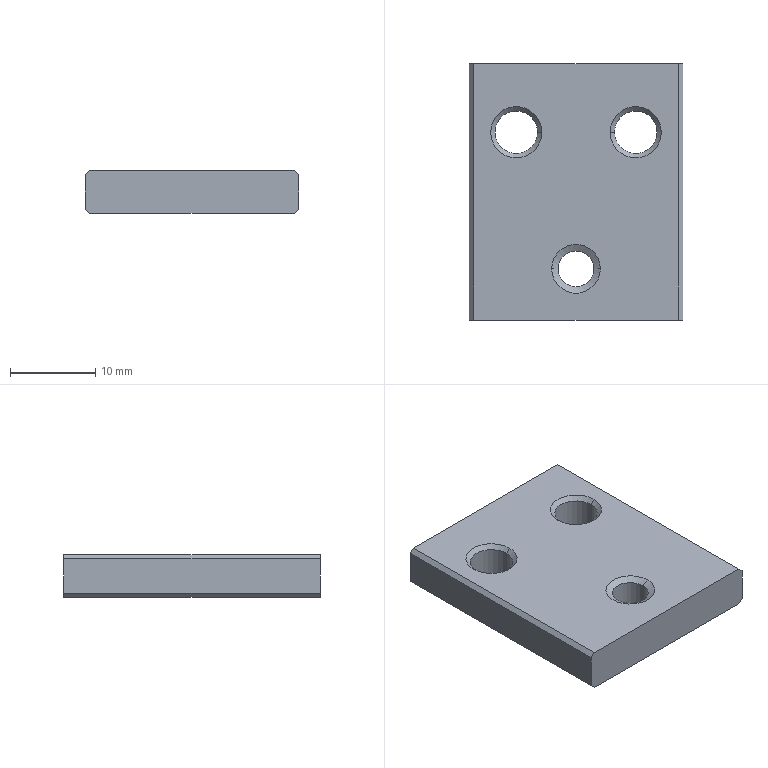Part | NX | 1 solid | 26 faces | box 25 x 30 x 5 mm | volume 3459 mm3 | plane 10 | cone 10 | cylinder 6 | commonest cylinder face diameters 5 x4 4.2 x2
STEP:
#1=CARTESIAN_POINT('',(-12.,-9.53,2.5));
#2=VERTEX_POINT('',#1);
#3=CARTESIAN_POINT('',(-12.,20.47,2.5));
#4=VERTEX_POINT('',#3);
#5=CARTESIAN_POINT('',(-12.,0.,2.5));
#6=DIRECTION('',(0.,1.,0.));
#7=VECTOR('',#6,1000.);
#8=LINE('',#5,#7);
#9=EDGE_CURVE('',#2,#4,#8,.T.);
#10=ORIENTED_EDGE('',*,*,#9,.F.);
#11=CARTESIAN_POINT('',(12.,-9.53,2.5));
#12=VERTEX_POINT('',#11);
#13=CARTESIAN_POINT('',(0.,-9.53,2.5));
#14=DIRECTION('',(1.,0.,0.));
#15=VECTOR('',#14,1000.);
#16=LINE('',#13,#15);
#17=EDGE_CURVE('',#2,#12,#16,.T.);
#18=ORIENTED_EDGE('',*,*,#17,.T.);
#19=CARTESIAN_POINT('',(12.,20.47,2.5));
#20=VERTEX_POINT('',#19);
#21=CARTESIAN_POINT('',(12.,0.,2.5));
#22=DIRECTION('',(0.,-1.,0.));
#23=VECTOR('',#22,1000.);
#24=LINE('',#21,#23);
#25=EDGE_CURVE('',#20,#12,#24,.T.);
#26=ORIENTED_EDGE('',*,*,#25,.F.);
#27=CARTESIAN_POINT('',(0.,20.47,2.5));
#28=DIRECTION('',(1.,0.,0.));
#29=VECTOR('',#28,1000.);
#30=LINE('',#27,#29);
#31=EDGE_CURVE('',#4,#20,#30,.T.);
#32=ORIENTED_EDGE('',*,*,#31,.F.);
#33=EDGE_LOOP('',(#10,#18,#26,#32));
#34=FACE_BOUND('',#33,.T.);
#35=CARTESIAN_POINT('',(-10.,12.47,2.5));
#36=VERTEX_POINT('',#35);
#37=CARTESIAN_POINT('',(-4.,12.47,2.5));
#38=VERTEX_POINT('',#37);
#39=CARTESIAN_POINT('',(-7.,12.47,2.5));
#40=DIRECTION('',(0.,0.,1.));
#41=DIRECTION('',(1.,0.,0.));
#42=AXIS2_PLACEMENT_3D('',#39,#40,#41);
#43=CIRCLE('',#42,3.);
#44=EDGE_CURVE('',#36,#38,#43,.T.);
#45=ORIENTED_EDGE('',*,*,#44,.F.);
#46=CARTESIAN_POINT('',(-7.,12.47,2.5));
#47=DIRECTION('',(0.,0.,1.));
#48=DIRECTION('',(1.,0.,0.));
#49=AXIS2_PLACEMENT_3D('',#46,#47,#48);
#50=CIRCLE('',#49,3.);
#51=EDGE_CURVE('',#38,#36,#50,.T.);
#52=ORIENTED_EDGE('',*,*,#51,.F.);
#53=EDGE_LOOP('',(#45,#52));
#54=FACE_BOUND('',#53,.T.);
#55=CARTESIAN_POINT('',(-2.86,-3.53,2.5));
#56=VERTEX_POINT('',#55);
#57=CARTESIAN_POINT('',(2.86,-3.53,2.5));
#58=VERTEX_POINT('',#57);
#59=CARTESIAN_POINT('',(0.,-3.53,2.5));
#60=DIRECTION('',(0.,0.,1.));
#61=DIRECTION('',(1.,0.,0.));
#62=AXIS2_PLACEMENT_3D('',#59,#60,#61);
#63=CIRCLE('',#62,2.86);
#64=EDGE_CURVE('',#56,#58,#63,.T.);
#65=ORIENTED_EDGE('',*,*,#64,.F.);
#66=CARTESIAN_POINT('',(0.,-3.53,2.5));
#67=DIRECTION('',(0.,0.,1.));
#68=DIRECTION('',(1.,0.,0.));
#69=AXIS2_PLACEMENT_3D('',#66,#67,#68);
#70=CIRCLE('',#69,2.86);
#71=EDGE_CURVE('',#58,#56,#70,.T.);
#72=ORIENTED_EDGE('',*,*,#71,.F.);
#73=EDGE_LOOP('',(#65,#72));
#74=FACE_BOUND('',#73,.T.);
#75=CARTESIAN_POINT('',(10.,12.47,2.5));
#76=VERTEX_POINT('',#75);
#77=CARTESIAN_POINT('',(4.,12.47,2.5));
#78=VERTEX_POINT('',#77);
#79=CARTESIAN_POINT('',(7.,12.47,2.5));
#80=DIRECTION('',(0.,0.,1.));
#81=DIRECTION('',(1.,0.,0.));
#82=AXIS2_PLACEMENT_3D('',#79,#80,#81);
#83=CIRCLE('',#82,3.);
#84=EDGE_CURVE('',#76,#78,#83,.T.);
#85=ORIENTED_EDGE('',*,*,#84,.F.);
#86=CARTESIAN_POINT('',(7.,12.47,2.5));
#87=DIRECTION('',(0.,0.,1.));
#88=DIRECTION('',(1.,0.,0.));
#89=AXIS2_PLACEMENT_3D('',#86,#87,#88);
#90=CIRCLE('',#89,3.);
#91=EDGE_CURVE('',#78,#76,#90,.T.);
#92=ORIENTED_EDGE('',*,*,#91,.F.);
#93=EDGE_LOOP('',(#85,#92));
#94=FACE_BOUND('',#93,.T.);
#95=CARTESIAN_POINT('',(0.,0.,2.5));
#96=DIRECTION('',(0.,0.,1.));
#97=DIRECTION('',(1.,0.,0.));
#98=AXIS2_PLACEMENT_3D('',#95,#96,#97);
#99=PLANE('',#98);
#100=ADVANCED_FACE('',(#34,#54,#74,#94),#99,.T.);
#101=ORIENTED_EDGE('',*,*,#17,.F.);
#102=CARTESIAN_POINT('',(-12.5,-9.53,2.));
#103=VERTEX_POINT('',#102);
#104=CARTESIAN_POINT('',(-14.5,-9.53,0.));
#105=DIRECTION('',(-0.7071,0.,-0.7071));
#106=VECTOR('',#105,1000.);
#107=LINE('',#104,#106);
#108=EDGE_CURVE('',#2,#103,#107,.T.);
#109=ORIENTED_EDGE('',*,*,#108,.T.);
#110=CARTESIAN_POINT('',(-12.5,-9.53,-2.));
#111=VERTEX_POINT('',#110);
#112=CARTESIAN_POINT('',(-12.5,-9.53,0.));
#113=DIRECTION('',(0.,0.,1.));
#114=VECTOR('',#113,1000.);
#115=LINE('',#112,#114);
#116=EDGE_CURVE('',#111,#103,#115,.T.);
#117=ORIENTED_EDGE('',*,*,#116,.F.);
#118=CARTESIAN_POINT('',(-12.,-9.53,-2.5));
#119=VERTEX_POINT('',#118);
#120=CARTESIAN_POINT('',(-14.5,-9.53,0.));
#121=DIRECTION('',(-0.7071,0.,0.7071));
#122=VECTOR('',#121,1000.);
#123=LINE('',#120,#122);
#124=EDGE_CURVE('',#119,#111,#123,.T.);
#125=ORIENTED_EDGE('',*,*,#124,.F.);
#126=CARTESIAN_POINT('',(12.,-9.53,-2.5));
#127=VERTEX_POINT('',#126);
#128=CARTESIAN_POINT('',(0.,-9.53,-2.5));
#129=DIRECTION('',(1.,0.,0.));
#130=VECTOR('',#129,1000.);
#131=LINE('',#128,#130);
#132=EDGE_CURVE('',#119,#127,#131,.T.);
#133=ORIENTED_EDGE('',*,*,#132,.T.);
#134=CARTESIAN_POINT('',(12.5,-9.53,-2.));
#135=VERTEX_POINT('',#134);
#136=CARTESIAN_POINT('',(14.5,-9.53,0.));
#137=DIRECTION('',(0.7071,0.,0.7071));
#138=VECTOR('',#137,1000.);
#139=LINE('',#136,#138);
#140=EDGE_CURVE('',#127,#135,#139,.T.);
#141=ORIENTED_EDGE('',*,*,#140,.T.);
#142=CARTESIAN_POINT('',(12.5,-9.53,2.));
#143=VERTEX_POINT('',#142);
#144=CARTESIAN_POINT('',(12.5,-9.53,0.));
#145=DIRECTION('',(0.,0.,-1.));
#146=VECTOR('',#145,1000.);
#147=LINE('',#144,#146);
#148=EDGE_CURVE('',#143,#135,#147,.T.);
#149=ORIENTED_EDGE('',*,*,#148,.F.);
#150=CARTESIAN_POINT('',(14.5,-9.53,0.));
#151=DIRECTION('',(-0.7071,0.,0.7071));
#152=VECTOR('',#151,1000.);
#153=LINE('',#150,#152);
#154=EDGE_CURVE('',#143,#12,#153,.T.);
#155=ORIENTED_EDGE('',*,*,#154,.T.);
#156=EDGE_LOOP('',(#101,#109,#117,#125,#133,#141,#149,#155));
#157=FACE_BOUND('',#156,.T.);
#158=CARTESIAN_POINT('',(179.5,-9.53,3.));
#159=DIRECTION('',(0.,1.,0.));
#160=DIRECTION('',(1.,0.,0.));
#161=AXIS2_PLACEMENT_3D('',#158,#159,#160);
#162=PLANE('',#161);
#163=ADVANCED_FACE('',(#157),#162,.F.);
#164=CARTESIAN_POINT('',(-12.,20.47,-2.5));
#165=VERTEX_POINT('',#164);
#166=CARTESIAN_POINT('',(12.,20.47,-2.5));
#167=VERTEX_POINT('',#166);
#168=CARTESIAN_POINT('',(0.,20.47,-2.5));
#169=DIRECTION('',(1.,0.,0.));
#170=VECTOR('',#169,1000.);
#171=LINE('',#168,#170);
#172=EDGE_CURVE('',#165,#167,#171,.T.);
#173=ORIENTED_EDGE('',*,*,#172,.F.);
#174=CARTESIAN_POINT('',(-12.5,20.47,-2.));
#175=VERTEX_POINT('',#174);
#176=CARTESIAN_POINT('',(-14.5,20.47,0.));
#177=DIRECTION('',(-0.7071,0.,0.7071));
#178=VECTOR('',#177,1000.);
#179=LINE('',#176,#178);
#180=EDGE_CURVE('',#165,#175,#179,.T.);
#181=ORIENTED_EDGE('',*,*,#180,.T.);
#182=CARTESIAN_POINT('',(-12.5,20.47,2.));
#183=VERTEX_POINT('',#182);
#184=CARTESIAN_POINT('',(-12.5,20.47,0.));
#185=DIRECTION('',(0.,0.,1.));
#186=VECTOR('',#185,1000.);
#187=LINE('',#184,#186);
#188=EDGE_CURVE('',#175,#183,#187,.T.);
#189=ORIENTED_EDGE('',*,*,#188,.T.);
#190=CARTESIAN_POINT('',(-14.5,20.47,0.));
#191=DIRECTION('',(0.7071,0.,0.7071));
#192=VECTOR('',#191,1000.);
#193=LINE('',#190,#192);
#194=EDGE_CURVE('',#183,#4,#193,.T.);
#195=ORIENTED_EDGE('',*,*,#194,.T.);
#196=ORIENTED_EDGE('',*,*,#31,.T.);
#197=CARTESIAN_POINT('',(12.5,20.47,2.));
#198=VERTEX_POINT('',#197);
#199=CARTESIAN_POINT('',(14.5,20.47,0.));
#200=DIRECTION('',(0.7071,0.,-0.7071));
#201=VECTOR('',#200,1000.);
#202=LINE('',#199,#201);
#203=EDGE_CURVE('',#20,#198,#202,.T.);
#204=ORIENTED_EDGE('',*,*,#203,.T.);
#205=CARTESIAN_POINT('',(12.5,20.47,-2.));
#206=VERTEX_POINT('',#205);
#207=CARTESIAN_POINT('',(12.5,20.47,0.));
#208=DIRECTION('',(0.,0.,-1.));
#209=VECTOR('',#208,1000.);
#210=LINE('',#207,#209);
#211=EDGE_CURVE('',#198,#206,#210,.T.);
#212=ORIENTED_EDGE('',*,*,#211,.T.);
#213=CARTESIAN_POINT('',(14.5,20.47,0.));
#214=DIRECTION('',(-0.7071,0.,-0.7071));
#215=VECTOR('',#214,1000.);
#216=LINE('',#213,#215);
#217=EDGE_CURVE('',#206,#167,#216,.T.);
#218=ORIENTED_EDGE('',*,*,#217,.T.);
#219=EDGE_LOOP('',(#173,#181,#189,#195,#196,#204,#212,#218));
#220=FACE_BOUND('',#219,.T.);
#221=CARTESIAN_POINT('',(-38.,20.47,-99.5));
#222=DIRECTION('',(0.,1.,0.));
#223=DIRECTION('',(1.,0.,0.));
#224=AXIS2_PLACEMENT_3D('',#221,#222,#223);
#225=PLANE('',#224);
#226=ADVANCED_FACE('',(#220),#225,.T.);
#227=CARTESIAN_POINT('',(12.5,0.,2.));
#228=DIRECTION('',(0.,1.,0.));
#229=VECTOR('',#228,1000.);
#230=LINE('',#227,#229);
#231=EDGE_CURVE('',#143,#198,#230,.T.);
#232=ORIENTED_EDGE('',*,*,#231,.F.);
#233=ORIENTED_EDGE('',*,*,#148,.T.);
#234=CARTESIAN_POINT('',(12.5,0.,-2.));
#235=DIRECTION('',(0.,-1.,0.));
#236=VECTOR('',#235,1000.);
#237=LINE('',#234,#236);
#238=EDGE_CURVE('',#206,#135,#237,.T.);
#239=ORIENTED_EDGE('',*,*,#238,.F.);
#240=ORIENTED_EDGE('',*,*,#211,.F.);
#241=EDGE_LOOP('',(#232,#233,#239,#240));
#242=FACE_BOUND('',#241,.T.);
#243=CARTESIAN_POINT('',(12.5,-20.5,-2.5));
#244=DIRECTION('',(1.,0.,0.));
#245=DIRECTION('',(0.,1.,0.));
#246=AXIS2_PLACEMENT_3D('',#243,#244,#245);
#247=PLANE('',#246);
#248=ADVANCED_FACE('',(#242),#247,.T.);
#249=ORIENTED_EDGE('',*,*,#140,.F.);
#250=CARTESIAN_POINT('',(12.,0.,-2.5));
#251=DIRECTION('',(0.,-1.,0.));
#252=VECTOR('',#251,1000.);
#253=LINE('',#250,#252);
#254=EDGE_CURVE('',#167,#127,#253,.T.);
#255=ORIENTED_EDGE('',*,*,#254,.F.);
#256=ORIENTED_EDGE('',*,*,#217,.F.);
#257=ORIENTED_EDGE('',*,*,#238,.T.);
#258=EDGE_LOOP('',(#249,#255,#256,#257));
#259=FACE_BOUND('',#258,.T.);
#260=CARTESIAN_POINT('',(12.25,0.,-2.25));
#261=DIRECTION('',(0.7071,0.,-0.7071));
#262=DIRECTION('',(0.,-1.,0.));
#263=AXIS2_PLACEMENT_3D('',#260,#261,#262);
#264=PLANE('',#263);
#265=ADVANCED_FACE('',(#259),#264,.T.);
#266=ORIENTED_EDGE('',*,*,#108,.F.);
#267=ORIENTED_EDGE('',*,*,#9,.T.);
#268=ORIENTED_EDGE('',*,*,#194,.F.);
#269=CARTESIAN_POINT('',(-12.5,0.,2.));
#270=DIRECTION('',(0.,-1.,0.));
#271=VECTOR('',#270,1000.);
#272=LINE('',#269,#271);
#273=EDGE_CURVE('',#183,#103,#272,.T.);
#274=ORIENTED_EDGE('',*,*,#273,.T.);
#275=EDGE_LOOP('',(#266,#267,#268,#274));
#276=FACE_BOUND('',#275,.T.);
#277=CARTESIAN_POINT('',(-12.25,0.,2.25));
#278=DIRECTION('',(-0.7071,0.,0.7071));
#279=DIRECTION('',(0.,1.,0.));
#280=AXIS2_PLACEMENT_3D('',#277,#278,#279);
#281=PLANE('',#280);
#282=ADVANCED_FACE('',(#276),#281,.T.);
#283=CARTESIAN_POINT('',(-9.5,12.47,2.));
#284=VERTEX_POINT('',#283);
#285=CARTESIAN_POINT('',(-4.5,12.47,2.));
#286=VERTEX_POINT('',#285);
#287=CARTESIAN_POINT('',(-7.,12.47,2.));
#288=DIRECTION('',(0.,0.,-1.));
#289=DIRECTION('',(-1.,0.,0.));
#290=AXIS2_PLACEMENT_3D('',#287,#288,#289);
#291=CIRCLE('',#290,2.5);
#292=EDGE_CURVE('',#284,#286,#291,.T.);
#293=ORIENTED_EDGE('',*,*,#292,.F.);
#294=CARTESIAN_POINT('',(-9.5,12.47,-2.));
#295=VERTEX_POINT('',#294);
#296=CARTESIAN_POINT('',(-9.5,12.47,2.5));
#297=DIRECTION('',(0.,0.,-1.));
#298=VECTOR('',#297,1000.);
#299=LINE('',#296,#298);
#300=EDGE_CURVE('',#295,#284,#299,.F.);
#301=ORIENTED_EDGE('',*,*,#300,.F.);
#302=CARTESIAN_POINT('',(-4.5,12.47,-2.));
#303=VERTEX_POINT('',#302);
#304=CARTESIAN_POINT('',(-7.,12.47,-2.));
#305=DIRECTION('',(0.,0.,-1.));
#306=DIRECTION('',(-1.,0.,0.));
#307=AXIS2_PLACEMENT_3D('',#304,#305,#306);
#308=CIRCLE('',#307,2.5);
#309=EDGE_CURVE('',#295,#303,#308,.T.);
#310=ORIENTED_EDGE('',*,*,#309,.T.);
#311=CARTESIAN_POINT('',(-4.5,12.47,2.5));
#312=DIRECTION('',(0.,0.,-1.));
#313=VECTOR('',#312,1000.);
#314=LINE('',#311,#313);
#315=EDGE_CURVE('',#303,#286,#314,.F.);
#316=ORIENTED_EDGE('',*,*,#315,.T.);
#317=EDGE_LOOP('',(#293,#301,#310,#316));
#318=FACE_BOUND('',#317,.T.);
#319=CARTESIAN_POINT('',(-7.,12.47,2.5));
#320=DIRECTION('',(0.,0.,-1.));
#321=DIRECTION('',(-1.,0.,0.));
#322=AXIS2_PLACEMENT_3D('',#319,#320,#321);
#323=CYLINDRICAL_SURFACE('',#322,2.5);
#324=ADVANCED_FACE('',(#318),#323,.F.);
#325=CARTESIAN_POINT('',(9.5,12.47,2.));
#326=VERTEX_POINT('',#325);
#327=CARTESIAN_POINT('',(4.5,12.47,2.));
#328=VERTEX_POINT('',#327);
#329=CARTESIAN_POINT('',(7.,12.47,2.));
#330=DIRECTION('',(0.,0.,-1.));
#331=DIRECTION('',(-1.,0.,0.));
#332=AXIS2_PLACEMENT_3D('',#329,#330,#331);
#333=CIRCLE('',#332,2.5);
#334=EDGE_CURVE('',#326,#328,#333,.T.);
#335=ORIENTED_EDGE('',*,*,#334,.F.);
#336=CARTESIAN_POINT('',(9.5,12.47,-2.));
#337=VERTEX_POINT('',#336);
#338=CARTESIAN_POINT('',(9.5,12.47,2.5));
#339=DIRECTION('',(0.,0.,-1.));
#340=VECTOR('',#339,1000.);
#341=LINE('',#338,#340);
#342=EDGE_CURVE('',#326,#337,#341,.T.);
#343=ORIENTED_EDGE('',*,*,#342,.T.);
#344=CARTESIAN_POINT('',(4.5,12.47,-2.));
#345=VERTEX_POINT('',#344);
#346=CARTESIAN_POINT('',(7.,12.47,-2.));
#347=DIRECTION('',(0.,0.,-1.));
#348=DIRECTION('',(-1.,0.,0.));
#349=AXIS2_PLACEMENT_3D('',#346,#347,#348);
#350=CIRCLE('',#349,2.5);
#351=EDGE_CURVE('',#337,#345,#350,.T.);
#352=ORIENTED_EDGE('',*,*,#351,.T.);
#353=CARTESIAN_POINT('',(4.5,12.47,2.5));
#354=DIRECTION('',(0.,0.,-1.));
#355=VECTOR('',#354,1000.);
#356=LINE('',#353,#355);
#357=EDGE_CURVE('',#328,#345,#356,.T.);
#358=ORIENTED_EDGE('',*,*,#357,.F.);
#359=EDGE_LOOP('',(#335,#343,#352,#358));
#360=FACE_BOUND('',#359,.T.);
#361=CARTESIAN_POINT('',(7.,12.47,2.5));
#362=DIRECTION('',(0.,0.,-1.));
#363=DIRECTION('',(-1.,0.,0.));
#364=AXIS2_PLACEMENT_3D('',#361,#362,#363);
#365=CYLINDRICAL_SURFACE('',#364,2.5);
#366=ADVANCED_FACE('',(#360),#365,.F.);
#367=ORIENTED_EDGE('',*,*,#231,.T.);
#368=ORIENTED_EDGE('',*,*,#203,.F.);
#369=ORIENTED_EDGE('',*,*,#25,.T.);
#370=ORIENTED_EDGE('',*,*,#154,.F.);
#371=EDGE_LOOP('',(#367,#368,#369,#370));
#372=FACE_BOUND('',#371,.T.);
#373=CARTESIAN_POINT('',(12.25,0.,2.25));
#374=DIRECTION('',(0.7071,0.,0.7071));
#375=DIRECTION('',(0.,-1.,0.));
#376=AXIS2_PLACEMENT_3D('',#373,#374,#375);
#377=PLANE('',#376);
#378=ADVANCED_FACE('',(#372),#377,.T.);
#379=ORIENTED_EDGE('',*,*,#116,.T.);
#380=ORIENTED_EDGE('',*,*,#273,.F.);
#381=ORIENTED_EDGE('',*,*,#188,.F.);
#382=CARTESIAN_POINT('',(-12.5,0.,-2.));
#383=DIRECTION('',(0.,-1.,0.));
#384=VECTOR('',#383,1000.);
#385=LINE('',#382,#384);
#386=EDGE_CURVE('',#175,#111,#385,.T.);
#387=ORIENTED_EDGE('',*,*,#386,.T.);
#388=EDGE_LOOP('',(#379,#380,#381,#387));
#389=FACE_BOUND('',#388,.T.);
#390=CARTESIAN_POINT('',(-12.5,20.5,-2.5));
#391=DIRECTION('',(-1.,0.,0.));
#392=DIRECTION('',(0.,0.,1.));
#393=AXIS2_PLACEMENT_3D('',#390,#391,#392);
#394=PLANE('',#393);
#395=ADVANCED_FACE('',(#389),#394,.T.);
#396=ORIENTED_EDGE('',*,*,#292,.T.);
#397=CARTESIAN_POINT('',(-4.,12.47,2.5));
#398=DIRECTION('',(0.7071,0.,0.7071));
#399=VECTOR('',#398,1000.);
#400=LINE('',#397,#399);
#401=EDGE_CURVE('',#286,#38,#400,.T.);
#402=ORIENTED_EDGE('',*,*,#401,.T.);
#403=ORIENTED_EDGE('',*,*,#51,.T.);
#404=CARTESIAN_POINT('',(-10.,12.47,2.5));
#405=DIRECTION('',(-0.7071,0.,0.7071));
#406=VECTOR('',#405,1000.);
#407=LINE('',#404,#406);
#408=EDGE_CURVE('',#284,#36,#407,.T.);
#409=ORIENTED_EDGE('',*,*,#408,.F.);
#410=EDGE_LOOP('',(#396,#402,#403,#409));
#411=FACE_BOUND('',#410,.T.);
#412=CARTESIAN_POINT('',(-7.,12.47,2.5));
#413=DIRECTION('',(0.,0.,1.));
#414=DIRECTION('',(1.,0.,0.));
#415=AXIS2_PLACEMENT_3D('',#412,#413,#414);
#416=CONICAL_SURFACE('',#415,3.,0.7854);
#417=ADVANCED_FACE('',(#411),#416,.F.);
#418=ORIENTED_EDGE('',*,*,#84,.T.);
#419=CARTESIAN_POINT('',(4.,12.47,2.5));
#420=DIRECTION('',(-0.7071,0.,0.7071));
#421=VECTOR('',#420,1000.);
#422=LINE('',#419,#421);
#423=EDGE_CURVE('',#78,#328,#422,.F.);
#424=ORIENTED_EDGE('',*,*,#423,.T.);
#425=CARTESIAN_POINT('',(7.,12.47,2.));
#426=DIRECTION('',(0.,0.,-1.));
#427=DIRECTION('',(-1.,0.,0.));
#428=AXIS2_PLACEMENT_3D('',#425,#426,#427);
#429=CIRCLE('',#428,2.5);
#430=EDGE_CURVE('',#328,#326,#429,.T.);
#431=ORIENTED_EDGE('',*,*,#430,.T.);
#432=CARTESIAN_POINT('',(10.,12.47,2.5));
#433=DIRECTION('',(0.7071,0.,0.7071));
#434=VECTOR('',#433,1000.);
#435=LINE('',#432,#434);
#436=EDGE_CURVE('',#76,#326,#435,.F.);
#437=ORIENTED_EDGE('',*,*,#436,.F.);
#438=EDGE_LOOP('',(#418,#424,#431,#437));
#439=FACE_BOUND('',#438,.T.);
#440=CARTESIAN_POINT('',(7.,12.47,2.5));
#441=DIRECTION('',(0.,0.,1.));
#442=DIRECTION('',(1.,0.,0.));
#443=AXIS2_PLACEMENT_3D('',#440,#441,#442);
#444=CONICAL_SURFACE('',#443,3.,0.7854);
#445=ADVANCED_FACE('',(#439),#444,.F.);
#446=CARTESIAN_POINT('',(10.,12.47,-2.5));
#447=VERTEX_POINT('',#446);
#448=CARTESIAN_POINT('',(4.,12.47,-2.5));
#449=VERTEX_POINT('',#448);
#450=CARTESIAN_POINT('',(7.,12.47,-2.5));
#451=DIRECTION('',(0.,0.,-1.));
#452=DIRECTION('',(-1.,0.,0.));
#453=AXIS2_PLACEMENT_3D('',#450,#451,#452);
#454=CIRCLE('',#453,3.);
#455=EDGE_CURVE('',#447,#449,#454,.T.);
#456=ORIENTED_EDGE('',*,*,#455,.T.);
#457=CARTESIAN_POINT('',(4.,12.47,-2.5));
#458=DIRECTION('',(-0.7071,0.,-0.7071));
#459=VECTOR('',#458,1000.);
#460=LINE('',#457,#459);
#461=EDGE_CURVE('',#449,#345,#460,.F.);
#462=ORIENTED_EDGE('',*,*,#461,.T.);
#463=ORIENTED_EDGE('',*,*,#351,.F.);
#464=CARTESIAN_POINT('',(10.,12.47,-2.5));
#465=DIRECTION('',(0.7071,0.,-0.7071));
#466=VECTOR('',#465,1000.);
#467=LINE('',#464,#466);
#468=EDGE_CURVE('',#447,#337,#467,.F.);
#469=ORIENTED_EDGE('',*,*,#468,.F.);
#470=EDGE_LOOP('',(#456,#462,#463,#469));
#471=FACE_BOUND('',#470,.T.);
#472=CARTESIAN_POINT('',(7.,12.47,-2.5));
#473=DIRECTION('',(0.,0.,-1.));
#474=DIRECTION('',(-1.,0.,0.));
#475=AXIS2_PLACEMENT_3D('',#472,#473,#474);
#476=CONICAL_SURFACE('',#475,3.,0.7854);
#477=ADVANCED_FACE('',(#471),#476,.F.);
#478=ORIENTED_EDGE('',*,*,#309,.F.);
#479=CARTESIAN_POINT('',(-10.,12.47,-2.5));
#480=VERTEX_POINT('',#479);
#481=CARTESIAN_POINT('',(-10.,12.47,-2.5));
#482=DIRECTION('',(-0.7071,0.,-0.7071));
#483=VECTOR('',#482,1000.);
#484=LINE('',#481,#483);
#485=EDGE_CURVE('',#480,#295,#484,.F.);
#486=ORIENTED_EDGE('',*,*,#485,.F.);
#487=CARTESIAN_POINT('',(-4.,12.47,-2.5));
#488=VERTEX_POINT('',#487);
#489=CARTESIAN_POINT('',(-7.,12.47,-2.5));
#490=DIRECTION('',(0.,0.,-1.));
#491=DIRECTION('',(-1.,0.,0.));
#492=AXIS2_PLACEMENT_3D('',#489,#490,#491);
#493=CIRCLE('',#492,3.);
#494=EDGE_CURVE('',#480,#488,#493,.T.);
#495=ORIENTED_EDGE('',*,*,#494,.T.);
#496=CARTESIAN_POINT('',(-4.,12.47,-2.5));
#497=DIRECTION('',(0.7071,0.,-0.7071));
#498=VECTOR('',#497,1000.);
#499=LINE('',#496,#498);
#500=EDGE_CURVE('',#488,#303,#499,.F.);
#501=ORIENTED_EDGE('',*,*,#500,.T.);
#502=EDGE_LOOP('',(#478,#486,#495,#501));
#503=FACE_BOUND('',#502,.T.);
#504=CARTESIAN_POINT('',(-7.,12.47,-2.5));
#505=DIRECTION('',(0.,0.,-1.));
#506=DIRECTION('',(-1.,0.,0.));
#507=AXIS2_PLACEMENT_3D('',#504,#505,#506);
#508=CONICAL_SURFACE('',#507,3.,0.7854);
#509=ADVANCED_FACE('',(#503),#508,.F.);
#510=CARTESIAN_POINT('',(-12.,0.,-2.5));
#511=DIRECTION('',(0.,1.,0.));
#512=VECTOR('',#511,1000.);
#513=LINE('',#510,#512);
#514=EDGE_CURVE('',#119,#165,#513,.T.);
#515=ORIENTED_EDGE('',*,*,#514,.F.);
#516=ORIENTED_EDGE('',*,*,#124,.T.);
#517=ORIENTED_EDGE('',*,*,#386,.F.);
#518=ORIENTED_EDGE('',*,*,#180,.F.);
#519=EDGE_LOOP('',(#515,#516,#517,#518));
#520=FACE_BOUND('',#519,.T.);
#521=CARTESIAN_POINT('',(-12.25,0.,-2.25));
#522=DIRECTION('',(-0.7071,0.,-0.7071));
#523=DIRECTION('',(-0.7071,0.,0.7071));
#524=AXIS2_PLACEMENT_3D('',#521,#522,#523);
#525=PLANE('',#524);
#526=ADVANCED_FACE('',(#520),#525,.T.);
#527=ORIENTED_EDGE('',*,*,#132,.F.);
#528=ORIENTED_EDGE('',*,*,#514,.T.);
#529=ORIENTED_EDGE('',*,*,#172,.T.);
#530=ORIENTED_EDGE('',*,*,#254,.T.);
#531=EDGE_LOOP('',(#527,#528,#529,#530));
#532=FACE_BOUND('',#531,.T.);
#533=ORIENTED_EDGE('',*,*,#494,.F.);
#534=CARTESIAN_POINT('',(-7.,12.47,-2.5));
#535=DIRECTION('',(0.,0.,-1.));
#536=DIRECTION('',(-1.,0.,0.));
#537=AXIS2_PLACEMENT_3D('',#534,#535,#536);
#538=CIRCLE('',#537,3.);
#539=EDGE_CURVE('',#488,#480,#538,.T.);
#540=ORIENTED_EDGE('',*,*,#539,.F.);
#541=EDGE_LOOP('',(#533,#540));
#542=FACE_BOUND('',#541,.T.);
#543=ORIENTED_EDGE('',*,*,#455,.F.);
#544=CARTESIAN_POINT('',(7.,12.47,-2.5));
#545=DIRECTION('',(0.,0.,-1.));
#546=DIRECTION('',(-1.,0.,0.));
#547=AXIS2_PLACEMENT_3D('',#544,#545,#546);
#548=CIRCLE('',#547,3.);
#549=EDGE_CURVE('',#449,#447,#548,.T.);
#550=ORIENTED_EDGE('',*,*,#549,.F.);
#551=EDGE_LOOP('',(#543,#550));
#552=FACE_BOUND('',#551,.T.);
#553=CARTESIAN_POINT('',(2.1,-3.53,-2.5));
#554=VERTEX_POINT('',#553);
#555=CARTESIAN_POINT('',(-2.1,-3.53,-2.5));
#556=VERTEX_POINT('',#555);
#557=CARTESIAN_POINT('',(0.,-3.53,-2.5));
#558=DIRECTION('',(0.,0.,1.));
#559=DIRECTION('',(1.,0.,0.));
#560=AXIS2_PLACEMENT_3D('',#557,#558,#559);
#561=CIRCLE('',#560,2.1);
#562=EDGE_CURVE('',#554,#556,#561,.T.);
#563=ORIENTED_EDGE('',*,*,#562,.T.);
#564=CARTESIAN_POINT('',(0.,-3.53,-2.5));
#565=DIRECTION('',(0.,0.,1.));
#566=DIRECTION('',(1.,0.,0.));
#567=AXIS2_PLACEMENT_3D('',#564,#565,#566);
#568=CIRCLE('',#567,2.1);
#569=EDGE_CURVE('',#556,#554,#568,.T.);
#570=ORIENTED_EDGE('',*,*,#569,.T.);
#571=EDGE_LOOP('',(#563,#570));
#572=FACE_BOUND('',#571,.T.);
#573=CARTESIAN_POINT('',(0.,0.,-2.5));
#574=DIRECTION('',(0.,0.,1.));
#575=DIRECTION('',(1.,0.,0.));
#576=AXIS2_PLACEMENT_3D('',#573,#574,#575);
#577=PLANE('',#576);
#578=ADVANCED_FACE('',(#532,#542,#552,#572),#577,.F.);
#579=CARTESIAN_POINT('',(2.1,-3.53,2.061));
#580=VERTEX_POINT('',#579);
#581=CARTESIAN_POINT('',(-2.1,-3.53,2.061));
#582=VERTEX_POINT('',#581);
#583=CARTESIAN_POINT('',(0.,-3.53,2.061));
#584=DIRECTION('',(0.,0.,1.));
#585=DIRECTION('',(1.,0.,0.));
#586=AXIS2_PLACEMENT_3D('',#583,#584,#585);
#587=CIRCLE('',#586,2.1);
#588=EDGE_CURVE('',#580,#582,#587,.T.);
#589=ORIENTED_EDGE('',*,*,#588,.T.);
#590=CARTESIAN_POINT('',(-2.1,-3.53,2.5));
#591=DIRECTION('',(0.,0.,1.));
#592=VECTOR('',#591,1000.);
#593=LINE('',#590,#592);
#594=EDGE_CURVE('',#556,#582,#593,.T.);
#595=ORIENTED_EDGE('',*,*,#594,.F.);
#596=ORIENTED_EDGE('',*,*,#562,.F.);
#597=CARTESIAN_POINT('',(2.1,-3.53,2.5));
#598=DIRECTION('',(0.,0.,1.));
#599=VECTOR('',#598,1000.);
#600=LINE('',#597,#599);
#601=EDGE_CURVE('',#554,#580,#600,.T.);
#602=ORIENTED_EDGE('',*,*,#601,.T.);
#603=EDGE_LOOP('',(#589,#595,#596,#602));
#604=FACE_BOUND('',#603,.T.);
#605=CARTESIAN_POINT('',(0.,-3.53,2.5));
#606=DIRECTION('',(0.,0.,1.));
#607=DIRECTION('',(1.,0.,0.));
#608=AXIS2_PLACEMENT_3D('',#605,#606,#607);
#609=CYLINDRICAL_SURFACE('',#608,2.1);
#610=ADVANCED_FACE('',(#604),#609,.F.);
#611=ORIENTED_EDGE('',*,*,#588,.F.);
#612=CARTESIAN_POINT('',(2.1,-3.53,2.061));
#613=DIRECTION('',(0.866,0.,0.5));
#614=VECTOR('',#613,1000.);
#615=LINE('',#612,#614);
#616=EDGE_CURVE('',#580,#58,#615,.T.);
#617=ORIENTED_EDGE('',*,*,#616,.T.);
#618=ORIENTED_EDGE('',*,*,#71,.T.);
#619=CARTESIAN_POINT('',(-2.1,-3.53,2.061));
#620=DIRECTION('',(-0.866,0.,0.5));
#621=VECTOR('',#620,1000.);
#622=LINE('',#619,#621);
#623=EDGE_CURVE('',#582,#56,#622,.T.);
#624=ORIENTED_EDGE('',*,*,#623,.F.);
#625=EDGE_LOOP('',(#611,#617,#618,#624));
#626=FACE_BOUND('',#625,.T.);
#627=CARTESIAN_POINT('',(0.,-3.53,2.061));
#628=DIRECTION('',(0.,0.,1.));
#629=DIRECTION('',(1.,0.,0.));
#630=AXIS2_PLACEMENT_3D('',#627,#628,#629);
#631=CONICAL_SURFACE('',#630,2.1,1.047);
#632=ADVANCED_FACE('',(#626),#631,.F.);
#633=ORIENTED_EDGE('',*,*,#300,.T.);
#634=CARTESIAN_POINT('',(-7.,12.47,2.));
#635=DIRECTION('',(0.,0.,-1.));
#636=DIRECTION('',(-1.,0.,0.));
#637=AXIS2_PLACEMENT_3D('',#634,#635,#636);
#638=CIRCLE('',#637,2.5);
#639=EDGE_CURVE('',#286,#284,#638,.T.);
#640=ORIENTED_EDGE('',*,*,#639,.F.);
#641=ORIENTED_EDGE('',*,*,#315,.F.);
#642=CARTESIAN_POINT('',(-7.,12.47,-2.));
#643=DIRECTION('',(0.,0.,-1.));
#644=DIRECTION('',(-1.,0.,0.));
#645=AXIS2_PLACEMENT_3D('',#642,#643,#644);
#646=CIRCLE('',#645,2.5);
#647=EDGE_CURVE('',#303,#295,#646,.T.);
#648=ORIENTED_EDGE('',*,*,#647,.T.);
#649=EDGE_LOOP('',(#633,#640,#641,#648));
#650=FACE_BOUND('',#649,.T.);
#651=CARTESIAN_POINT('',(-7.,12.47,2.5));
#652=DIRECTION('',(0.,0.,-1.));
#653=DIRECTION('',(-1.,0.,0.));
#654=AXIS2_PLACEMENT_3D('',#651,#652,#653);
#655=CYLINDRICAL_SURFACE('',#654,2.5);
#656=ADVANCED_FACE('',(#650),#655,.F.);
#657=ORIENTED_EDGE('',*,*,#64,.T.);
#658=ORIENTED_EDGE('',*,*,#616,.F.);
#659=CARTESIAN_POINT('',(0.,-3.53,2.061));
#660=DIRECTION('',(0.,0.,1.));
#661=DIRECTION('',(1.,0.,0.));
#662=AXIS2_PLACEMENT_3D('',#659,#660,#661);
#663=CIRCLE('',#662,2.1);
#664=EDGE_CURVE('',#582,#580,#663,.T.);
#665=ORIENTED_EDGE('',*,*,#664,.F.);
#666=ORIENTED_EDGE('',*,*,#623,.T.);
#667=EDGE_LOOP('',(#657,#658,#665,#666));
#668=FACE_BOUND('',#667,.T.);
#669=CARTESIAN_POINT('',(0.,-3.53,2.061));
#670=DIRECTION('',(0.,0.,1.));
#671=DIRECTION('',(1.,0.,0.));
#672=AXIS2_PLACEMENT_3D('',#669,#670,#671);
#673=CONICAL_SURFACE('',#672,2.1,1.047);
#674=ADVANCED_FACE('',(#668),#673,.F.);
#675=ORIENTED_EDGE('',*,*,#485,.T.);
#676=ORIENTED_EDGE('',*,*,#647,.F.);
#677=ORIENTED_EDGE('',*,*,#500,.F.);
#678=ORIENTED_EDGE('',*,*,#539,.T.);
#679=EDGE_LOOP('',(#675,#676,#677,#678));
#680=FACE_BOUND('',#679,.T.);
#681=CARTESIAN_POINT('',(-7.,12.47,-2.5));
#682=DIRECTION('',(0.,0.,-1.));
#683=DIRECTION('',(-1.,0.,0.));
#684=AXIS2_PLACEMENT_3D('',#681,#682,#683);
#685=CONICAL_SURFACE('',#684,3.,0.7854);
#686=ADVANCED_FACE('',(#680),#685,.F.);
#687=ORIENTED_EDGE('',*,*,#601,.F.);
#688=ORIENTED_EDGE('',*,*,#569,.F.);
#689=ORIENTED_EDGE('',*,*,#594,.T.);
#690=ORIENTED_EDGE('',*,*,#664,.T.);
#691=EDGE_LOOP('',(#687,#688,#689,#690));
#692=FACE_BOUND('',#691,.T.);
#693=CARTESIAN_POINT('',(0.,-3.53,2.5));
#694=DIRECTION('',(0.,0.,1.));
#695=DIRECTION('',(1.,0.,0.));
#696=AXIS2_PLACEMENT_3D('',#693,#694,#695);
#697=CYLINDRICAL_SURFACE('',#696,2.1);
#698=ADVANCED_FACE('',(#692),#697,.F.);
#699=ORIENTED_EDGE('',*,*,#334,.T.);
#700=ORIENTED_EDGE('',*,*,#423,.F.);
#701=ORIENTED_EDGE('',*,*,#91,.T.);
#702=ORIENTED_EDGE('',*,*,#436,.T.);
#703=EDGE_LOOP('',(#699,#700,#701,#702));
#704=FACE_BOUND('',#703,.T.);
#705=CARTESIAN_POINT('',(7.,12.47,2.5));
#706=DIRECTION('',(0.,0.,1.));
#707=DIRECTION('',(1.,0.,0.));
#708=AXIS2_PLACEMENT_3D('',#705,#706,#707);
#709=CONICAL_SURFACE('',#708,3.,0.7854);
#710=ADVANCED_FACE('',(#704),#709,.F.);
#711=CARTESIAN_POINT('',(7.,12.47,-2.));
#712=DIRECTION('',(0.,0.,-1.));
#713=DIRECTION('',(-1.,0.,0.));
#714=AXIS2_PLACEMENT_3D('',#711,#712,#713);
#715=CIRCLE('',#714,2.5);
#716=EDGE_CURVE('',#345,#337,#715,.T.);
#717=ORIENTED_EDGE('',*,*,#716,.T.);
#718=ORIENTED_EDGE('',*,*,#342,.F.);
#719=ORIENTED_EDGE('',*,*,#430,.F.);
#720=ORIENTED_EDGE('',*,*,#357,.T.);
#721=EDGE_LOOP('',(#717,#718,#719,#720));
#722=FACE_BOUND('',#721,.T.);
#723=CARTESIAN_POINT('',(7.,12.47,2.5));
#724=DIRECTION('',(0.,0.,-1.));
#725=DIRECTION('',(-1.,0.,0.));
#726=AXIS2_PLACEMENT_3D('',#723,#724,#725);
#727=CYLINDRICAL_SURFACE('',#726,2.5);
#728=ADVANCED_FACE('',(#722),#727,.F.);
#729=ORIENTED_EDGE('',*,*,#716,.F.);
#730=ORIENTED_EDGE('',*,*,#461,.F.);
#731=ORIENTED_EDGE('',*,*,#549,.T.);
#732=ORIENTED_EDGE('',*,*,#468,.T.);
#733=EDGE_LOOP('',(#729,#730,#731,#732));
#734=FACE_BOUND('',#733,.T.);
#735=CARTESIAN_POINT('',(7.,12.47,-2.5));
#736=DIRECTION('',(0.,0.,-1.));
#737=DIRECTION('',(-1.,0.,0.));
#738=AXIS2_PLACEMENT_3D('',#735,#736,#737);
#739=CONICAL_SURFACE('',#738,3.,0.7854);
#740=ADVANCED_FACE('',(#734),#739,.F.);
#741=ORIENTED_EDGE('',*,*,#44,.T.);
#742=ORIENTED_EDGE('',*,*,#401,.F.);
#743=ORIENTED_EDGE('',*,*,#639,.T.);
#744=ORIENTED_EDGE('',*,*,#408,.T.);
#745=EDGE_LOOP('',(#741,#742,#743,#744));
#746=FACE_BOUND('',#745,.T.);
#747=CARTESIAN_POINT('',(-7.,12.47,2.5));
#748=DIRECTION('',(0.,0.,1.));
#749=DIRECTION('',(1.,0.,0.));
#750=AXIS2_PLACEMENT_3D('',#747,#748,#749);
#751=CONICAL_SURFACE('',#750,3.,0.7854);
#752=ADVANCED_FACE('',(#746),#751,.F.);
#753=CLOSED_SHELL('',(#100,#163,#226,#248,#265,#282,#324,#366,#378,#395,#417,#445,#477,#509,#526,#578,#610,#632,#656,#674,#686,#698,#710,#728,#740,#752));
#754=MANIFOLD_SOLID_BREP('',#753);
#755=(LENGTH_UNIT()NAMED_UNIT(*)SI_UNIT(.MILLI.,.METRE.));
#756=UNCERTAINTY_MEASURE_WITH_UNIT(LENGTH_MEASURE(0.00001),#755,'','');
#757=(NAMED_UNIT(*)PLANE_ANGLE_UNIT()SI_UNIT($,.RADIAN.));
#758=(NAMED_UNIT(*)SI_UNIT($,.STERADIAN.)SOLID_ANGLE_UNIT());
#759=(GEOMETRIC_REPRESENTATION_CONTEXT(3)GLOBAL_UNCERTAINTY_ASSIGNED_CONTEXT((#756))GLOBAL_UNIT_ASSIGNED_CONTEXT((#755,#757,#758))REPRESENTATION_CONTEXT('',''));
#760=ADVANCED_BREP_SHAPE_REPRESENTATION('',(#754),#759);